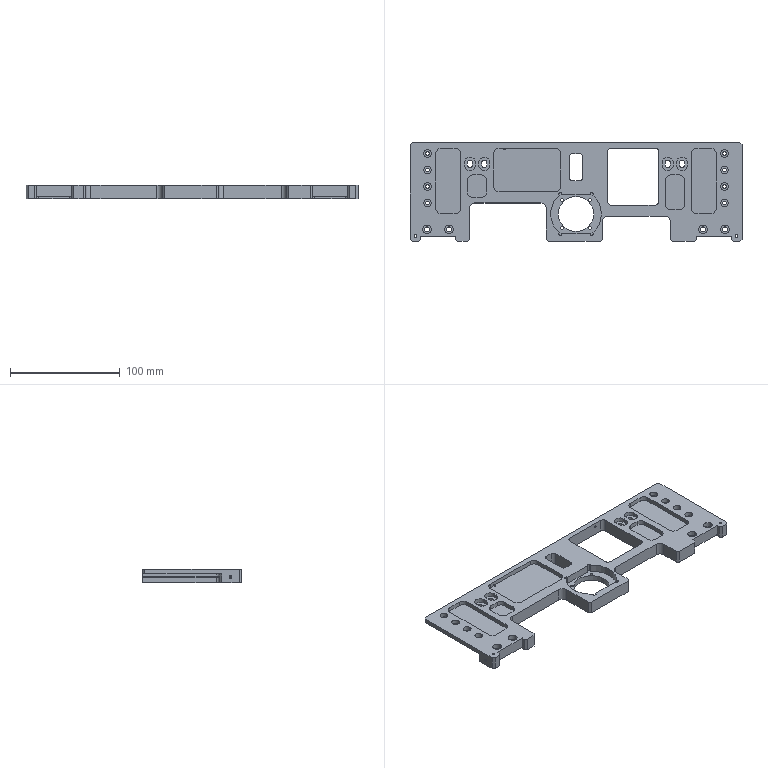Part | NX | features BREP 1 | 1 solid | 339 faces | box 302 x 90 x 12 mm | volume 154751 mm3 | cylinder 169 | plane 159 | cone 11 | commonest cylinder face diameters 10 x52 2.5 x16 3.4 x16 4.5 x16 7 x16 6 x14